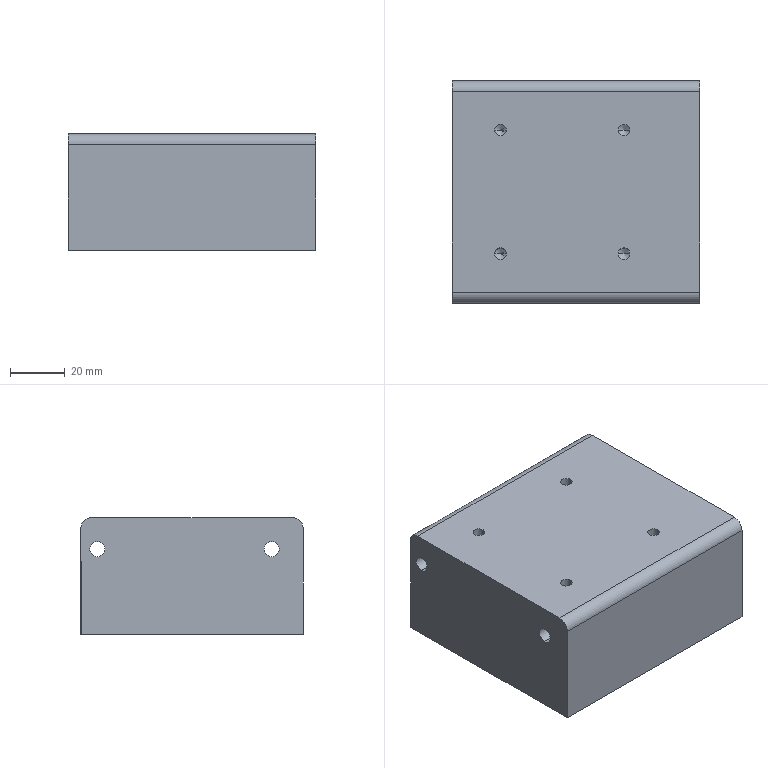Part | STEP file | FFH80-GY-003B^FFH85-PL-M75-B3-01_three-axis module | 1 solid | 45 faces | box 90 x 81 x 42.5 mm | volume 303221 mm3 | cylinder 23 | plane 12 | cone 10 | commonest cylinder face diameters 4.2 x8 5.5 x4 9 x4 2.5 x2 3 x2 8 x2
STEP:
#1=CARTESIAN_POINT('',(84.,34.5,14.25));
#2=VERTEX_POINT('',#1);
#3=CARTESIAN_POINT('',(84.,34.5,5.25));
#4=VERTEX_POINT('',#3);
#5=CARTESIAN_POINT('',(84.,34.5,9.75));
#6=DIRECTION('',(1.,0.,0.));
#7=DIRECTION('',(0.,0.,-1.));
#8=AXIS2_PLACEMENT_3D('',#5,#6,#7);
#9=CIRCLE('',#8,4.5);
#10=EDGE_CURVE('',#2,#4,#9,.T.);
#11=ORIENTED_EDGE('',*,*,#10,.F.);
#12=CARTESIAN_POINT('',(90.,34.5,14.25));
#13=VERTEX_POINT('',#12);
#14=CARTESIAN_POINT('',(90.,34.5,14.25));
#15=DIRECTION('',(1.,0.,0.));
#16=VECTOR('',#15,1000.);
#17=LINE('',#14,#16);
#18=EDGE_CURVE('',#2,#13,#17,.T.);
#19=ORIENTED_EDGE('',*,*,#18,.T.);
#20=CARTESIAN_POINT('',(90.,34.5,5.25));
#21=VERTEX_POINT('',#20);
#22=CARTESIAN_POINT('',(90.,34.5,9.75));
#23=DIRECTION('',(1.,0.,0.));
#24=DIRECTION('',(0.,0.,-1.));
#25=AXIS2_PLACEMENT_3D('',#22,#23,#24);
#26=CIRCLE('',#25,4.5);
#27=EDGE_CURVE('',#13,#21,#26,.T.);
#28=ORIENTED_EDGE('',*,*,#27,.T.);
#29=CARTESIAN_POINT('',(90.,34.5,5.25));
#30=DIRECTION('',(1.,0.,0.));
#31=VECTOR('',#30,1000.);
#32=LINE('',#29,#31);
#33=EDGE_CURVE('',#4,#21,#32,.T.);
#34=ORIENTED_EDGE('',*,*,#33,.F.);
#35=EDGE_LOOP('',(#11,#19,#28,#34));
#36=FACE_OUTER_BOUND('',#35,.T.);
#37=CARTESIAN_POINT('',(90.,34.5,9.75));
#38=DIRECTION('',(1.,0.,0.));
#39=DIRECTION('',(0.,0.,-1.));
#40=AXIS2_PLACEMENT_3D('',#37,#38,#39);
#41=CYLINDRICAL_SURFACE('',#40,4.5);
#42=ADVANCED_FACE('',(#36),#41,.F.);
#43=CARTESIAN_POINT('',(84.,-29.,14.25));
#44=VERTEX_POINT('',#43);
#45=CARTESIAN_POINT('',(84.,-29.,5.25));
#46=VERTEX_POINT('',#45);
#47=CARTESIAN_POINT('',(84.,-29.,9.75));
#48=DIRECTION('',(1.,0.,0.));
#49=DIRECTION('',(0.,0.,-1.));
#50=AXIS2_PLACEMENT_3D('',#47,#48,#49);
#51=CIRCLE('',#50,4.5);
#52=EDGE_CURVE('',#44,#46,#51,.T.);
#53=ORIENTED_EDGE('',*,*,#52,.F.);
#54=CARTESIAN_POINT('',(90.,-29.,14.25));
#55=VERTEX_POINT('',#54);
#56=CARTESIAN_POINT('',(90.,-29.,14.25));
#57=DIRECTION('',(1.,0.,0.));
#58=VECTOR('',#57,1000.);
#59=LINE('',#56,#58);
#60=EDGE_CURVE('',#44,#55,#59,.T.);
#61=ORIENTED_EDGE('',*,*,#60,.T.);
#62=CARTESIAN_POINT('',(90.,-29.,5.25));
#63=VERTEX_POINT('',#62);
#64=CARTESIAN_POINT('',(90.,-29.,9.75));
#65=DIRECTION('',(1.,0.,0.));
#66=DIRECTION('',(0.,0.,-1.));
#67=AXIS2_PLACEMENT_3D('',#64,#65,#66);
#68=CIRCLE('',#67,4.5);
#69=EDGE_CURVE('',#55,#63,#68,.T.);
#70=ORIENTED_EDGE('',*,*,#69,.T.);
#71=CARTESIAN_POINT('',(90.,-29.,5.25));
#72=DIRECTION('',(1.,0.,0.));
#73=VECTOR('',#72,1000.);
#74=LINE('',#71,#73);
#75=EDGE_CURVE('',#46,#63,#74,.T.);
#76=ORIENTED_EDGE('',*,*,#75,.F.);
#77=EDGE_LOOP('',(#53,#61,#70,#76));
#78=FACE_OUTER_BOUND('',#77,.T.);
#79=CARTESIAN_POINT('',(90.,-29.,9.75));
#80=DIRECTION('',(1.,0.,0.));
#81=DIRECTION('',(0.,0.,-1.));
#82=AXIS2_PLACEMENT_3D('',#79,#80,#81);
#83=CYLINDRICAL_SURFACE('',#82,4.5);
#84=ADVANCED_FACE('',(#78),#83,.F.);
#85=CARTESIAN_POINT('',(0.,34.5,12.5));
#86=VERTEX_POINT('',#85);
#87=CARTESIAN_POINT('',(0.,34.5,7.));
#88=VERTEX_POINT('',#87);
#89=CARTESIAN_POINT('',(0.,34.5,9.75));
#90=DIRECTION('',(1.,0.,0.));
#91=DIRECTION('',(0.,0.,-1.));
#92=AXIS2_PLACEMENT_3D('',#89,#90,#91);
#93=CIRCLE('',#92,2.75);
#94=EDGE_CURVE('',#86,#88,#93,.T.);
#95=ORIENTED_EDGE('',*,*,#94,.F.);
#96=CARTESIAN_POINT('',(84.,34.5,12.5));
#97=VERTEX_POINT('',#96);
#98=CARTESIAN_POINT('',(90.,34.5,12.5));
#99=DIRECTION('',(1.,0.,0.));
#100=VECTOR('',#99,1000.);
#101=LINE('',#98,#100);
#102=EDGE_CURVE('',#86,#97,#101,.T.);
#103=ORIENTED_EDGE('',*,*,#102,.T.);
#104=CARTESIAN_POINT('',(84.,34.5,7.));
#105=VERTEX_POINT('',#104);
#106=CARTESIAN_POINT('',(84.,34.5,9.75));
#107=DIRECTION('',(-1.,0.,0.));
#108=DIRECTION('',(0.,0.,-1.));
#109=AXIS2_PLACEMENT_3D('',#106,#107,#108);
#110=CIRCLE('',#109,2.75);
#111=EDGE_CURVE('',#105,#97,#110,.T.);
#112=ORIENTED_EDGE('',*,*,#111,.F.);
#113=CARTESIAN_POINT('',(90.,34.5,7.));
#114=DIRECTION('',(1.,0.,0.));
#115=VECTOR('',#114,1000.);
#116=LINE('',#113,#115);
#117=EDGE_CURVE('',#88,#105,#116,.T.);
#118=ORIENTED_EDGE('',*,*,#117,.F.);
#119=EDGE_LOOP('',(#95,#103,#112,#118));
#120=FACE_OUTER_BOUND('',#119,.T.);
#121=CARTESIAN_POINT('',(90.,34.5,9.75));
#122=DIRECTION('',(1.,0.,0.));
#123=DIRECTION('',(0.,0.,-1.));
#124=AXIS2_PLACEMENT_3D('',#121,#122,#123);
#125=CYLINDRICAL_SURFACE('',#124,2.75);
#126=ADVANCED_FACE('',(#120),#125,.F.);
#127=CARTESIAN_POINT('',(0.,-29.,12.5));
#128=VERTEX_POINT('',#127);
#129=CARTESIAN_POINT('',(0.,-29.,7.));
#130=VERTEX_POINT('',#129);
#131=CARTESIAN_POINT('',(0.,-29.,9.75));
#132=DIRECTION('',(1.,0.,0.));
#133=DIRECTION('',(0.,0.,-1.));
#134=AXIS2_PLACEMENT_3D('',#131,#132,#133);
#135=CIRCLE('',#134,2.75);
#136=EDGE_CURVE('',#128,#130,#135,.T.);
#137=ORIENTED_EDGE('',*,*,#136,.F.);
#138=CARTESIAN_POINT('',(84.,-29.,12.5));
#139=VERTEX_POINT('',#138);
#140=CARTESIAN_POINT('',(90.,-29.,12.5));
#141=DIRECTION('',(1.,0.,0.));
#142=VECTOR('',#141,1000.);
#143=LINE('',#140,#142);
#144=EDGE_CURVE('',#128,#139,#143,.T.);
#145=ORIENTED_EDGE('',*,*,#144,.T.);
#146=CARTESIAN_POINT('',(84.,-29.,7.));
#147=VERTEX_POINT('',#146);
#148=CARTESIAN_POINT('',(84.,-29.,9.75));
#149=DIRECTION('',(-1.,0.,0.));
#150=DIRECTION('',(0.,0.,-1.));
#151=AXIS2_PLACEMENT_3D('',#148,#149,#150);
#152=CIRCLE('',#151,2.75);
#153=EDGE_CURVE('',#147,#139,#152,.T.);
#154=ORIENTED_EDGE('',*,*,#153,.F.);
#155=CARTESIAN_POINT('',(90.,-29.,7.));
#156=DIRECTION('',(1.,0.,0.));
#157=VECTOR('',#156,1000.);
#158=LINE('',#155,#157);
#159=EDGE_CURVE('',#130,#147,#158,.T.);
#160=ORIENTED_EDGE('',*,*,#159,.F.);
#161=EDGE_LOOP('',(#137,#145,#154,#160));
#162=FACE_OUTER_BOUND('',#161,.T.);
#163=CARTESIAN_POINT('',(90.,-29.,9.75));
#164=DIRECTION('',(1.,0.,0.));
#165=DIRECTION('',(0.,0.,-1.));
#166=AXIS2_PLACEMENT_3D('',#163,#164,#165);
#167=CYLINDRICAL_SURFACE('',#166,2.75);
#168=ADVANCED_FACE('',(#162),#167,.F.);
#169=CARTESIAN_POINT('',(6.,34.2,-6.75));
#170=VERTEX_POINT('',#169);
#171=CARTESIAN_POINT('',(6.,34.2,-3.75));
#172=VERTEX_POINT('',#171);
#173=CARTESIAN_POINT('',(6.,34.2,-5.25));
#174=DIRECTION('',(0.,1.,0.));
#175=DIRECTION('',(0.,0.,1.));
#176=AXIS2_PLACEMENT_3D('',#173,#174,#175);
#177=CIRCLE('',#176,1.5);
#178=EDGE_CURVE('',#170,#172,#177,.T.);
#179=ORIENTED_EDGE('',*,*,#178,.F.);
#180=CARTESIAN_POINT('',(6.,40.2,-6.75));
#181=VERTEX_POINT('',#180);
#182=CARTESIAN_POINT('',(6.,40.2,-6.75));
#183=DIRECTION('',(0.,1.,0.));
#184=VECTOR('',#183,1000.);
#185=LINE('',#182,#184);
#186=EDGE_CURVE('',#170,#181,#185,.T.);
#187=ORIENTED_EDGE('',*,*,#186,.T.);
#188=CARTESIAN_POINT('',(6.,40.2,-3.75));
#189=VERTEX_POINT('',#188);
#190=CARTESIAN_POINT('',(6.,40.2,-5.25));
#191=DIRECTION('',(0.,-1.,0.));
#192=DIRECTION('',(0.,0.,1.));
#193=AXIS2_PLACEMENT_3D('',#190,#191,#192);
#194=CIRCLE('',#193,1.5);
#195=EDGE_CURVE('',#189,#181,#194,.T.);
#196=ORIENTED_EDGE('',*,*,#195,.F.);
#197=CARTESIAN_POINT('',(6.,40.2,-3.75));
#198=DIRECTION('',(0.,1.,0.));
#199=VECTOR('',#198,1000.);
#200=LINE('',#197,#199);
#201=EDGE_CURVE('',#172,#189,#200,.T.);
#202=ORIENTED_EDGE('',*,*,#201,.F.);
#203=EDGE_LOOP('',(#179,#187,#196,#202));
#204=FACE_OUTER_BOUND('',#203,.T.);
#205=CARTESIAN_POINT('',(6.,40.2,-5.25));
#206=DIRECTION('',(0.,1.,0.));
#207=DIRECTION('',(0.,0.,1.));
#208=AXIS2_PLACEMENT_3D('',#205,#206,#207);
#209=CYLINDRICAL_SURFACE('',#208,1.5);
#210=ADVANCED_FACE('',(#204),#209,.F.);
#211=CARTESIAN_POINT('',(60.4,22.5,2.25));
#212=VERTEX_POINT('',#211);
#213=CARTESIAN_POINT('',(64.6,22.5,2.25));
#214=VERTEX_POINT('',#213);
#215=CARTESIAN_POINT('',(62.5,22.5,2.25));
#216=DIRECTION('',(0.,0.,1.));
#217=DIRECTION('',(1.,0.,0.));
#218=AXIS2_PLACEMENT_3D('',#215,#216,#217);
#219=CIRCLE('',#218,2.1);
#220=EDGE_CURVE('',#212,#214,#219,.T.);
#221=ORIENTED_EDGE('',*,*,#220,.F.);
#222=CARTESIAN_POINT('',(60.4,22.5,21.25));
#223=VERTEX_POINT('',#222);
#224=CARTESIAN_POINT('',(60.4,22.5,21.25));
#225=DIRECTION('',(0.,0.,1.));
#226=VECTOR('',#225,1000.);
#227=LINE('',#224,#226);
#228=EDGE_CURVE('',#212,#223,#227,.T.);
#229=ORIENTED_EDGE('',*,*,#228,.T.);
#230=CARTESIAN_POINT('',(64.6,22.5,21.25));
#231=VERTEX_POINT('',#230);
#232=CARTESIAN_POINT('',(62.5,22.5,21.25));
#233=DIRECTION('',(0.,0.,1.));
#234=DIRECTION('',(1.,0.,0.));
#235=AXIS2_PLACEMENT_3D('',#232,#233,#234);
#236=CIRCLE('',#235,2.1);
#237=EDGE_CURVE('',#223,#231,#236,.T.);
#238=ORIENTED_EDGE('',*,*,#237,.T.);
#239=CARTESIAN_POINT('',(64.6,22.5,21.25));
#240=DIRECTION('',(0.,0.,1.));
#241=VECTOR('',#240,1000.);
#242=LINE('',#239,#241);
#243=EDGE_CURVE('',#214,#231,#242,.T.);
#244=ORIENTED_EDGE('',*,*,#243,.F.);
#245=EDGE_LOOP('',(#221,#229,#238,#244));
#246=FACE_OUTER_BOUND('',#245,.T.);
#247=CARTESIAN_POINT('',(62.5,22.5,21.25));
#248=DIRECTION('',(0.,0.,1.));
#249=DIRECTION('',(1.,0.,0.));
#250=AXIS2_PLACEMENT_3D('',#247,#248,#249);
#251=CYLINDRICAL_SURFACE('',#250,2.1);
#252=ADVANCED_FACE('',(#246),#251,.F.);
#253=CARTESIAN_POINT('',(15.4,22.5,2.25));
#254=VERTEX_POINT('',#253);
#255=CARTESIAN_POINT('',(19.6,22.5,2.25));
#256=VERTEX_POINT('',#255);
#257=CARTESIAN_POINT('',(17.5,22.5,2.25));
#258=DIRECTION('',(0.,0.,1.));
#259=DIRECTION('',(1.,0.,0.));
#260=AXIS2_PLACEMENT_3D('',#257,#258,#259);
#261=CIRCLE('',#260,2.1);
#262=EDGE_CURVE('',#254,#256,#261,.T.);
#263=ORIENTED_EDGE('',*,*,#262,.F.);
#264=CARTESIAN_POINT('',(15.4,22.5,21.25));
#265=VERTEX_POINT('',#264);
#266=CARTESIAN_POINT('',(15.4,22.5,21.25));
#267=DIRECTION('',(0.,0.,1.));
#268=VECTOR('',#267,1000.);
#269=LINE('',#266,#268);
#270=EDGE_CURVE('',#254,#265,#269,.T.);
#271=ORIENTED_EDGE('',*,*,#270,.T.);
#272=CARTESIAN_POINT('',(19.6,22.5,21.25));
#273=VERTEX_POINT('',#272);
#274=CARTESIAN_POINT('',(17.5,22.5,21.25));
#275=DIRECTION('',(0.,0.,1.));
#276=DIRECTION('',(1.,0.,0.));
#277=AXIS2_PLACEMENT_3D('',#274,#275,#276);
#278=CIRCLE('',#277,2.1);
#279=EDGE_CURVE('',#265,#273,#278,.T.);
#280=ORIENTED_EDGE('',*,*,#279,.T.);
#281=CARTESIAN_POINT('',(19.6,22.5,21.25));
#282=DIRECTION('',(0.,0.,1.));
#283=VECTOR('',#282,1000.);
#284=LINE('',#281,#283);
#285=EDGE_CURVE('',#256,#273,#284,.T.);
#286=ORIENTED_EDGE('',*,*,#285,.F.);
#287=EDGE_LOOP('',(#263,#271,#280,#286));
#288=FACE_OUTER_BOUND('',#287,.T.);
#289=CARTESIAN_POINT('',(17.5,22.5,21.25));
#290=DIRECTION('',(0.,0.,1.));
#291=DIRECTION('',(1.,0.,0.));
#292=AXIS2_PLACEMENT_3D('',#289,#290,#291);
#293=CYLINDRICAL_SURFACE('',#292,2.1);
#294=ADVANCED_FACE('',(#288),#293,.F.);
#295=CARTESIAN_POINT('',(60.4,-22.5,2.25));
#296=VERTEX_POINT('',#295);
#297=CARTESIAN_POINT('',(64.6,-22.5,2.25));
#298=VERTEX_POINT('',#297);
#299=CARTESIAN_POINT('',(62.5,-22.5,2.25));
#300=DIRECTION('',(0.,0.,1.));
#301=DIRECTION('',(1.,0.,0.));
#302=AXIS2_PLACEMENT_3D('',#299,#300,#301);
#303=CIRCLE('',#302,2.1);
#304=EDGE_CURVE('',#296,#298,#303,.T.);
#305=ORIENTED_EDGE('',*,*,#304,.F.);
#306=CARTESIAN_POINT('',(60.4,-22.5,21.25));
#307=VERTEX_POINT('',#306);
#308=CARTESIAN_POINT('',(60.4,-22.5,21.25));
#309=DIRECTION('',(0.,0.,1.));
#310=VECTOR('',#309,1000.);
#311=LINE('',#308,#310);
#312=EDGE_CURVE('',#296,#307,#311,.T.);
#313=ORIENTED_EDGE('',*,*,#312,.T.);
#314=CARTESIAN_POINT('',(64.6,-22.5,21.25));
#315=VERTEX_POINT('',#314);
#316=CARTESIAN_POINT('',(62.5,-22.5,21.25));
#317=DIRECTION('',(0.,0.,1.));
#318=DIRECTION('',(1.,0.,0.));
#319=AXIS2_PLACEMENT_3D('',#316,#317,#318);
#320=CIRCLE('',#319,2.1);
#321=EDGE_CURVE('',#307,#315,#320,.T.);
#322=ORIENTED_EDGE('',*,*,#321,.T.);
#323=CARTESIAN_POINT('',(64.6,-22.5,21.25));
#324=DIRECTION('',(0.,0.,1.));
#325=VECTOR('',#324,1000.);
#326=LINE('',#323,#325);
#327=EDGE_CURVE('',#298,#315,#326,.T.);
#328=ORIENTED_EDGE('',*,*,#327,.F.);
#329=EDGE_LOOP('',(#305,#313,#322,#328));
#330=FACE_OUTER_BOUND('',#329,.T.);
#331=CARTESIAN_POINT('',(62.5,-22.5,21.25));
#332=DIRECTION('',(0.,0.,1.));
#333=DIRECTION('',(1.,0.,0.));
#334=AXIS2_PLACEMENT_3D('',#331,#332,#333);
#335=CYLINDRICAL_SURFACE('',#334,2.1);
#336=ADVANCED_FACE('',(#330),#335,.F.);
#337=CARTESIAN_POINT('',(15.4,-22.5,2.25));
#338=VERTEX_POINT('',#337);
#339=CARTESIAN_POINT('',(19.6,-22.5,2.25));
#340=VERTEX_POINT('',#339);
#341=CARTESIAN_POINT('',(17.5,-22.5,2.25));
#342=DIRECTION('',(0.,0.,1.));
#343=DIRECTION('',(1.,0.,0.));
#344=AXIS2_PLACEMENT_3D('',#341,#342,#343);
#345=CIRCLE('',#344,2.1);
#346=EDGE_CURVE('',#338,#340,#345,.T.);
#347=ORIENTED_EDGE('',*,*,#346,.F.);
#348=CARTESIAN_POINT('',(15.4,-22.5,21.25));
#349=VERTEX_POINT('',#348);
#350=CARTESIAN_POINT('',(15.4,-22.5,21.25));
#351=DIRECTION('',(0.,0.,1.));
#352=VECTOR('',#351,1000.);
#353=LINE('',#350,#352);
#354=EDGE_CURVE('',#338,#349,#353,.T.);
#355=ORIENTED_EDGE('',*,*,#354,.T.);
#356=CARTESIAN_POINT('',(19.6,-22.5,21.25));
#357=VERTEX_POINT('',#356);
#358=CARTESIAN_POINT('',(17.5,-22.5,21.25));
#359=DIRECTION('',(0.,0.,1.));
#360=DIRECTION('',(1.,0.,0.));
#361=AXIS2_PLACEMENT_3D('',#358,#359,#360);
#362=CIRCLE('',#361,2.1);
#363=EDGE_CURVE('',#349,#357,#362,.T.);
#364=ORIENTED_EDGE('',*,*,#363,.T.);
#365=CARTESIAN_POINT('',(19.6,-22.5,21.25));
#366=DIRECTION('',(0.,0.,1.));
#367=VECTOR('',#366,1000.);
#368=LINE('',#365,#367);
#369=EDGE_CURVE('',#340,#357,#368,.T.);
#370=ORIENTED_EDGE('',*,*,#369,.F.);
#371=EDGE_LOOP('',(#347,#355,#364,#370));
#372=FACE_OUTER_BOUND('',#371,.T.);
#373=CARTESIAN_POINT('',(17.5,-22.5,21.25));
#374=DIRECTION('',(0.,0.,1.));
#375=DIRECTION('',(1.,0.,0.));
#376=AXIS2_PLACEMENT_3D('',#373,#374,#375);
#377=CYLINDRICAL_SURFACE('',#376,2.1);
#378=ADVANCED_FACE('',(#372),#377,.F.);
#379=CARTESIAN_POINT('',(62.5,22.5,0.9882));
#380=VERTEX_POINT('',#379);
#381=CARTESIAN_POINT('',(64.6,22.5,2.25));
#382=DIRECTION('',(0.8572,0.,0.515));
#383=VECTOR('',#382,1000.);
#384=LINE('',#381,#383);
#385=EDGE_CURVE('',#380,#214,#384,.T.);
#386=ORIENTED_EDGE('',*,*,#385,.F.);
#387=CARTESIAN_POINT('',(60.4,22.5,2.25));
#388=DIRECTION('',(-0.8572,0.,0.515));
#389=VECTOR('',#388,1000.);
#390=LINE('',#387,#389);
#391=EDGE_CURVE('',#380,#212,#390,.T.);
#392=ORIENTED_EDGE('',*,*,#391,.T.);
#393=ORIENTED_EDGE('',*,*,#220,.T.);
#394=EDGE_LOOP('',(#386,#392,#393));
#395=FACE_OUTER_BOUND('',#394,.T.);
#396=CARTESIAN_POINT('',(62.5,22.5,2.25));
#397=DIRECTION('',(0.,0.,1.));
#398=DIRECTION('',(1.,0.,0.));
#399=AXIS2_PLACEMENT_3D('',#396,#397,#398);
#400=CONICAL_SURFACE('',#399,2.1,1.03);
#401=ADVANCED_FACE('',(#395),#400,.F.);
#402=CARTESIAN_POINT('',(17.5,22.5,0.9882));
#403=VERTEX_POINT('',#402);
#404=CARTESIAN_POINT('',(19.6,22.5,2.25));
#405=DIRECTION('',(0.8572,0.,0.515));
#406=VECTOR('',#405,1000.);
#407=LINE('',#404,#406);
#408=EDGE_CURVE('',#403,#256,#407,.T.);
#409=ORIENTED_EDGE('',*,*,#408,.F.);
#410=CARTESIAN_POINT('',(15.4,22.5,2.25));
#411=DIRECTION('',(-0.8572,0.,0.515));
#412=VECTOR('',#411,1000.);
#413=LINE('',#410,#412);
#414=EDGE_CURVE('',#403,#254,#413,.T.);
#415=ORIENTED_EDGE('',*,*,#414,.T.);
#416=ORIENTED_EDGE('',*,*,#262,.T.);
#417=EDGE_LOOP('',(#409,#415,#416));
#418=FACE_OUTER_BOUND('',#417,.T.);
#419=CARTESIAN_POINT('',(17.5,22.5,2.25));
#420=DIRECTION('',(0.,0.,1.));
#421=DIRECTION('',(1.,0.,0.));
#422=AXIS2_PLACEMENT_3D('',#419,#420,#421);
#423=CONICAL_SURFACE('',#422,2.1,1.03);
#424=ADVANCED_FACE('',(#418),#423,.F.);
#425=CARTESIAN_POINT('',(62.5,-22.5,0.9882));
#426=VERTEX_POINT('',#425);
#427=CARTESIAN_POINT('',(64.6,-22.5,2.25));
#428=DIRECTION('',(0.8572,0.,0.515));
#429=VECTOR('',#428,1000.);
#430=LINE('',#427,#429);
#431=EDGE_CURVE('',#426,#298,#430,.T.);
#432=ORIENTED_EDGE('',*,*,#431,.F.);
#433=CARTESIAN_POINT('',(60.4,-22.5,2.25));
#434=DIRECTION('',(-0.8572,0.,0.515));
#435=VECTOR('',#434,1000.);
#436=LINE('',#433,#435);
#437=EDGE_CURVE('',#426,#296,#436,.T.);
#438=ORIENTED_EDGE('',*,*,#437,.T.);
#439=ORIENTED_EDGE('',*,*,#304,.T.);
#440=EDGE_LOOP('',(#432,#438,#439));
#441=FACE_OUTER_BOUND('',#440,.T.);
#442=CARTESIAN_POINT('',(62.5,-22.5,2.25));
#443=DIRECTION('',(0.,0.,1.));
#444=DIRECTION('',(1.,0.,0.));
#445=AXIS2_PLACEMENT_3D('',#442,#443,#444);
#446=CONICAL_SURFACE('',#445,2.1,1.03);
#447=ADVANCED_FACE('',(#441),#446,.F.);
#448=CARTESIAN_POINT('',(17.5,-22.5,0.9882));
#449=VERTEX_POINT('',#448);
#450=CARTESIAN_POINT('',(19.6,-22.5,2.25));
#451=DIRECTION('',(0.8572,0.,0.515));
#452=VECTOR('',#451,1000.);
#453=LINE('',#450,#452);
#454=EDGE_CURVE('',#449,#340,#453,.T.);
#455=ORIENTED_EDGE('',*,*,#454,.F.);
#456=CARTESIAN_POINT('',(15.4,-22.5,2.25));
#457=DIRECTION('',(-0.8572,0.,0.515));
#458=VECTOR('',#457,1000.);
#459=LINE('',#456,#458);
#460=EDGE_CURVE('',#449,#338,#459,.T.);
#461=ORIENTED_EDGE('',*,*,#460,.T.);
#462=ORIENTED_EDGE('',*,*,#346,.T.);
#463=EDGE_LOOP('',(#455,#461,#462));
#464=FACE_OUTER_BOUND('',#463,.T.);
#465=CARTESIAN_POINT('',(17.5,-22.5,2.25));
#466=DIRECTION('',(0.,0.,1.));
#467=DIRECTION('',(1.,0.,0.));
#468=AXIS2_PLACEMENT_3D('',#465,#466,#467);
#469=CONICAL_SURFACE('',#468,2.1,1.03);
#470=ADVANCED_FACE('',(#464),#469,.F.);
#471=CARTESIAN_POINT('',(6.,31.7,-6.5));
#472=VERTEX_POINT('',#471);
#473=CARTESIAN_POINT('',(6.,31.7,-4.));
#474=VERTEX_POINT('',#473);
#475=CARTESIAN_POINT('',(6.,31.7,-5.25));
#476=DIRECTION('',(0.,1.,0.));
#477=DIRECTION('',(0.,0.,1.));
#478=AXIS2_PLACEMENT_3D('',#475,#476,#477);
#479=CIRCLE('',#478,1.25);
#480=EDGE_CURVE('',#472,#474,#479,.T.);
#481=ORIENTED_EDGE('',*,*,#480,.F.);
#482=CARTESIAN_POINT('',(6.,34.2,-6.5));
#483=VERTEX_POINT('',#482);
#484=CARTESIAN_POINT('',(6.,40.2,-6.5));
#485=DIRECTION('',(0.,1.,0.));
#486=VECTOR('',#485,1000.);
#487=LINE('',#484,#486);
#488=EDGE_CURVE('',#472,#483,#487,.T.);
#489=ORIENTED_EDGE('',*,*,#488,.T.);
#490=CARTESIAN_POINT('',(6.,34.2,-4.));
#491=VERTEX_POINT('',#490);
#492=CARTESIAN_POINT('',(6.,34.2,-5.25));
#493=DIRECTION('',(0.,1.,0.));
#494=DIRECTION('',(0.,0.,1.));
#495=AXIS2_PLACEMENT_3D('',#492,#493,#494);
#496=CIRCLE('',#495,1.25);
#497=EDGE_CURVE('',#483,#491,#496,.T.);
#498=ORIENTED_EDGE('',*,*,#497,.T.);
#499=CARTESIAN_POINT('',(6.,40.2,-4.));
#500=DIRECTION('',(0.,1.,0.));
#501=VECTOR('',#500,1000.);
#502=LINE('',#499,#501);
#503=EDGE_CURVE('',#474,#491,#502,.T.);
#504=ORIENTED_EDGE('',*,*,#503,.F.);
#505=EDGE_LOOP('',(#481,#489,#498,#504));
#506=FACE_OUTER_BOUND('',#505,.T.);
#507=CARTESIAN_POINT('',(6.,40.2,-5.25));
#508=DIRECTION('',(0.,1.,0.));
#509=DIRECTION('',(0.,0.,1.));
#510=AXIS2_PLACEMENT_3D('',#507,#508,#509);
#511=CYLINDRICAL_SURFACE('',#510,1.25);
#512=ADVANCED_FACE('',(#506),#511,.F.);
#513=CARTESIAN_POINT('',(6.,30.949,-5.25));
#514=VERTEX_POINT('',#513);
#515=CARTESIAN_POINT('',(6.,31.7,-4.));
#516=DIRECTION('',(0.,0.515,0.8572));
#517=VECTOR('',#516,1000.);
#518=LINE('',#515,#517);
#519=EDGE_CURVE('',#514,#474,#518,.T.);
#520=ORIENTED_EDGE('',*,*,#519,.F.);
#521=CARTESIAN_POINT('',(6.,31.7,-6.5));
#522=DIRECTION('',(0.,0.515,-0.8572));
#523=VECTOR('',#522,1000.);
#524=LINE('',#521,#523);
#525=EDGE_CURVE('',#514,#472,#524,.T.);
#526=ORIENTED_EDGE('',*,*,#525,.T.);
#527=ORIENTED_EDGE('',*,*,#480,.T.);
#528=EDGE_LOOP('',(#520,#526,#527));
#529=FACE_OUTER_BOUND('',#528,.T.);
#530=CARTESIAN_POINT('',(6.,31.7,-5.25));
#531=DIRECTION('',(0.,1.,0.));
#532=DIRECTION('',(0.,0.,1.));
#533=AXIS2_PLACEMENT_3D('',#530,#531,#532);
#534=CONICAL_SURFACE('',#533,1.25,1.03);
#535=ADVANCED_FACE('',(#529),#534,.F.);
#536=CARTESIAN_POINT('',(90.,40.5,-21.25));
#537=VERTEX_POINT('',#536);
#538=CARTESIAN_POINT('',(12.5,40.5,-21.25));
#539=VERTEX_POINT('',#538);
#540=CARTESIAN_POINT('',(90.,40.5,-21.25));
#541=DIRECTION('',(-1.,0.,0.));
#542=VECTOR('',#541,1000.);
#543=LINE('',#540,#542);
#544=EDGE_CURVE('',#537,#539,#543,.T.);
#545=ORIENTED_EDGE('',*,*,#544,.F.);
#546=CARTESIAN_POINT('',(90.,-40.5,-21.25));
#547=VERTEX_POINT('',#546);
#548=CARTESIAN_POINT('',(90.,40.5,-21.25));
#549=DIRECTION('',(0.,1.,0.));
#550=VECTOR('',#549,1000.);
#551=LINE('',#548,#550);
#552=EDGE_CURVE('',#547,#537,#551,.T.);
#553=ORIENTED_EDGE('',*,*,#552,.F.);
#554=CARTESIAN_POINT('',(0.,-40.5,-21.25));
#555=VERTEX_POINT('',#554);
#556=CARTESIAN_POINT('',(90.,-40.5,-21.25));
#557=DIRECTION('',(1.,0.,0.));
#558=VECTOR('',#557,1000.);
#559=LINE('',#556,#558);
#560=EDGE_CURVE('',#555,#547,#559,.T.);
#561=ORIENTED_EDGE('',*,*,#560,.F.);
#562=CARTESIAN_POINT('',(0.,40.2,-21.25));
#563=VERTEX_POINT('',#562);
#564=CARTESIAN_POINT('',(0.,40.5,-21.25));
#565=DIRECTION('',(0.,-1.,0.));
#566=VECTOR('',#565,1000.);
#567=LINE('',#564,#566);
#568=EDGE_CURVE('',#563,#555,#567,.T.);
#569=ORIENTED_EDGE('',*,*,#568,.F.);
#570=CARTESIAN_POINT('',(12.5,40.2,-21.25));
#571=VERTEX_POINT('',#570);
#572=CARTESIAN_POINT('',(90.,40.2,-21.25));
#573=DIRECTION('',(-1.,0.,0.));
#574=VECTOR('',#573,1000.);
#575=LINE('',#572,#574);
#576=EDGE_CURVE('',#571,#563,#575,.T.);
#577=ORIENTED_EDGE('',*,*,#576,.F.);
#578=CARTESIAN_POINT('',(12.5,40.2,-21.25));
#579=DIRECTION('',(0.,1.,0.));
#580=VECTOR('',#579,1000.);
#581=LINE('',#578,#580);
#582=EDGE_CURVE('',#571,#539,#581,.T.);
#583=ORIENTED_EDGE('',*,*,#582,.T.);
#584=EDGE_LOOP('',(#545,#553,#561,#569,#577,#583));
#585=FACE_OUTER_BOUND('',#584,.T.);
#586=CARTESIAN_POINT('',(90.,40.5,-21.25));
#587=DIRECTION('',(0.,0.,1.));
#588=DIRECTION('',(0.,-1.,0.));
#589=AXIS2_PLACEMENT_3D('',#586,#587,#588);
#590=PLANE('',#589);
#591=ADVANCED_FACE('',(#585),#590,.F.);
#592=CARTESIAN_POINT('',(90.,40.5,17.25));
#593=VERTEX_POINT('',#592);
#594=CARTESIAN_POINT('',(90.,40.5,-21.25));
#595=DIRECTION('',(0.,0.,1.));
#596=VECTOR('',#595,1000.);
#597=LINE('',#594,#596);
#598=EDGE_CURVE('',#537,#593,#597,.T.);
#599=ORIENTED_EDGE('',*,*,#598,.F.);
#600=ORIENTED_EDGE('',*,*,#544,.T.);
#601=CARTESIAN_POINT('',(12.5,40.5,3.25));
#602=VERTEX_POINT('',#601);
#603=CARTESIAN_POINT('',(12.5,40.5,-21.25));
#604=DIRECTION('',(0.,0.,-1.));
#605=VECTOR('',#604,1000.);
#606=LINE('',#603,#605);
#607=EDGE_CURVE('',#602,#539,#606,.T.);
#608=ORIENTED_EDGE('',*,*,#607,.F.);
#609=CARTESIAN_POINT('',(10.5,40.5,5.25));
#610=VERTEX_POINT('',#609);
#611=CARTESIAN_POINT('',(10.5,40.5,3.25));
#612=DIRECTION('',(0.,1.,0.));
#613=DIRECTION('',(0.,0.,-1.));
#614=AXIS2_PLACEMENT_3D('',#611,#612,#613);
#615=CIRCLE('',#614,2.);
#616=EDGE_CURVE('',#610,#602,#615,.T.);
#617=ORIENTED_EDGE('',*,*,#616,.F.);
#618=CARTESIAN_POINT('',(0.,40.5,5.25));
#619=VERTEX_POINT('',#618);
#620=CARTESIAN_POINT('',(90.,40.5,5.25));
#621=DIRECTION('',(1.,0.,0.));
#622=VECTOR('',#621,1000.);
#623=LINE('',#620,#622);
#624=EDGE_CURVE('',#619,#610,#623,.T.);
#625=ORIENTED_EDGE('',*,*,#624,.F.);
#626=CARTESIAN_POINT('',(0.,40.5,17.25));
#627=VERTEX_POINT('',#626);
#628=CARTESIAN_POINT('',(0.,40.5,-21.25));
#629=DIRECTION('',(0.,0.,-1.));
#630=VECTOR('',#629,1000.);
#631=LINE('',#628,#630);
#632=EDGE_CURVE('',#627,#619,#631,.T.);
#633=ORIENTED_EDGE('',*,*,#632,.F.);
#634=CARTESIAN_POINT('',(90.,40.5,17.25));
#635=DIRECTION('',(-1.,0.,0.));
#636=VECTOR('',#635,1000.);
#637=LINE('',#634,#636);
#638=EDGE_CURVE('',#593,#627,#637,.T.);
#639=ORIENTED_EDGE('',*,*,#638,.F.);
#640=EDGE_LOOP('',(#599,#600,#608,#617,#625,#633,#639));
#641=FACE_OUTER_BOUND('',#640,.T.);
#642=CARTESIAN_POINT('',(90.,40.5,-21.25));
#643=DIRECTION('',(0.,-1.,0.));
#644=DIRECTION('',(0.,0.,-1.));
#645=AXIS2_PLACEMENT_3D('',#642,#643,#644);
#646=PLANE('',#645);
#647=ADVANCED_FACE('',(#641),#646,.F.);
#648=CARTESIAN_POINT('',(90.,34.5,9.75));
#649=DIRECTION('',(1.,0.,0.));
#650=DIRECTION('',(0.,0.,-1.));
#651=AXIS2_PLACEMENT_3D('',#648,#649,#650);
#652=CIRCLE('',#651,4.5);
#653=EDGE_CURVE('',#21,#13,#652,.T.);
#654=ORIENTED_EDGE('',*,*,#653,.F.);
#655=ORIENTED_EDGE('',*,*,#27,.F.);
#656=EDGE_LOOP('',(#654,#655));
#657=FACE_BOUND('',#656,.T.);
#658=CARTESIAN_POINT('',(90.,-29.,9.75));
#659=DIRECTION('',(1.,0.,0.));
#660=DIRECTION('',(0.,0.,-1.));
#661=AXIS2_PLACEMENT_3D('',#658,#659,#660);
#662=CIRCLE('',#661,4.5);
#663=EDGE_CURVE('',#63,#55,#662,.T.);
#664=ORIENTED_EDGE('',*,*,#663,.F.);
#665=ORIENTED_EDGE('',*,*,#69,.F.);
#666=EDGE_LOOP('',(#664,#665));
#667=FACE_BOUND('',#666,.T.);
#668=CARTESIAN_POINT('',(90.,-40.5,17.25));
#669=VERTEX_POINT('',#668);
#670=CARTESIAN_POINT('',(90.,-40.5,0.));
#671=DIRECTION('',(0.,0.,1.));
#672=VECTOR('',#671,1000.);
#673=LINE('',#670,#672);
#674=EDGE_CURVE('',#547,#669,#673,.T.);
#675=ORIENTED_EDGE('',*,*,#674,.F.);
#676=ORIENTED_EDGE('',*,*,#552,.T.);
#677=ORIENTED_EDGE('',*,*,#598,.T.);
#678=CARTESIAN_POINT('',(90.,36.5,21.25));
#679=VERTEX_POINT('',#678);
#680=CARTESIAN_POINT('',(90.,36.5,17.25));
#681=DIRECTION('',(-1.,0.,0.));
#682=DIRECTION('',(0.,0.,1.));
#683=AXIS2_PLACEMENT_3D('',#680,#681,#682);
#684=CIRCLE('',#683,4.);
#685=EDGE_CURVE('',#679,#593,#684,.T.);
#686=ORIENTED_EDGE('',*,*,#685,.F.);
#687=CARTESIAN_POINT('',(90.,-36.5,21.25));
#688=VERTEX_POINT('',#687);
#689=CARTESIAN_POINT('',(90.,0.,21.25));
#690=DIRECTION('',(0.,1.,0.));
#691=VECTOR('',#690,1000.);
#692=LINE('',#689,#691);
#693=EDGE_CURVE('',#688,#679,#692,.T.);
#694=ORIENTED_EDGE('',*,*,#693,.F.);
#695=CARTESIAN_POINT('',(90.,-36.5,17.25));
#696=DIRECTION('',(-1.,0.,0.));
#697=DIRECTION('',(0.,0.,1.));
#698=AXIS2_PLACEMENT_3D('',#695,#696,#697);
#699=CIRCLE('',#698,4.);
#700=EDGE_CURVE('',#669,#688,#699,.T.);
#701=ORIENTED_EDGE('',*,*,#700,.F.);
#702=EDGE_LOOP('',(#675,#676,#677,#686,#694,#701));
#703=FACE_OUTER_BOUND('',#702,.T.);
#704=CARTESIAN_POINT('',(90.,0.,0.));
#705=DIRECTION('',(-1.,0.,0.));
#706=DIRECTION('',(0.,0.,1.));
#707=AXIS2_PLACEMENT_3D('',#704,#705,#706);
#708=PLANE('',#707);
#709=ADVANCED_FACE('',(#657,#667,#703),#708,.F.);
#710=CARTESIAN_POINT('',(0.,-40.5,17.25));
#711=VERTEX_POINT('',#710);
#712=CARTESIAN_POINT('',(0.,-40.5,-21.25));
#713=DIRECTION('',(0.,0.,1.));
#714=VECTOR('',#713,1000.);
#715=LINE('',#712,#714);
#716=EDGE_CURVE('',#555,#711,#715,.T.);
#717=ORIENTED_EDGE('',*,*,#716,.F.);
#718=ORIENTED_EDGE('',*,*,#560,.T.);
#719=ORIENTED_EDGE('',*,*,#674,.T.);
#720=CARTESIAN_POINT('',(90.,-40.5,17.25));
#721=DIRECTION('',(1.,0.,0.));
#722=VECTOR('',#721,1000.);
#723=LINE('',#720,#722);
#724=EDGE_CURVE('',#711,#669,#723,.T.);
#725=ORIENTED_EDGE('',*,*,#724,.F.);
#726=EDGE_LOOP('',(#717,#718,#719,#725));
#727=FACE_OUTER_BOUND('',#726,.T.);
#728=CARTESIAN_POINT('',(90.,-40.5,-21.25));
#729=DIRECTION('',(0.,1.,0.));
#730=DIRECTION('',(0.,0.,1.));
#731=AXIS2_PLACEMENT_3D('',#728,#729,#730);
#732=PLANE('',#731);
#733=ADVANCED_FACE('',(#727),#732,.F.);
#734=ORIENTED_EDGE('',*,*,#632,.T.);
#735=CARTESIAN_POINT('',(0.,40.2,5.25));
#736=VERTEX_POINT('',#735);
#737=CARTESIAN_POINT('',(0.,0.,5.25));
#738=DIRECTION('',(0.,-1.,0.));
#739=VECTOR('',#738,1000.);
#740=LINE('',#737,#739);
#741=EDGE_CURVE('',#619,#736,#740,.T.);
#742=ORIENTED_EDGE('',*,*,#741,.T.);
#743=CARTESIAN_POINT('',(0.,40.2,0.));
#744=DIRECTION('',(0.,0.,-1.));
#745=VECTOR('',#744,1000.);
#746=LINE('',#743,#745);
#747=EDGE_CURVE('',#736,#563,#746,.T.);
#748=ORIENTED_EDGE('',*,*,#747,.T.);
#749=ORIENTED_EDGE('',*,*,#568,.T.);
#750=ORIENTED_EDGE('',*,*,#716,.T.);
#751=CARTESIAN_POINT('',(0.,-36.5,21.25));
#752=VERTEX_POINT('',#751);
#753=CARTESIAN_POINT('',(0.,-36.5,17.25));
#754=DIRECTION('',(-1.,0.,0.));
#755=DIRECTION('',(0.,0.,1.));
#756=AXIS2_PLACEMENT_3D('',#753,#754,#755);
#757=CIRCLE('',#756,4.);
#758=EDGE_CURVE('',#711,#752,#757,.T.);
#759=ORIENTED_EDGE('',*,*,#758,.T.);
#760=CARTESIAN_POINT('',(0.,36.5,21.25));
#761=VERTEX_POINT('',#760);
#762=CARTESIAN_POINT('',(0.,0.,21.25));
#763=DIRECTION('',(0.,1.,0.));
#764=VECTOR('',#763,1000.);
#765=LINE('',#762,#764);
#766=EDGE_CURVE('',#752,#761,#765,.T.);
#767=ORIENTED_EDGE('',*,*,#766,.T.);
#768=CARTESIAN_POINT('',(0.,36.5,17.25));
#769=DIRECTION('',(-1.,0.,0.));
#770=DIRECTION('',(0.,0.,1.));
#771=AXIS2_PLACEMENT_3D('',#768,#769,#770);
#772=CIRCLE('',#771,4.);
#773=EDGE_CURVE('',#761,#627,#772,.T.);
#774=ORIENTED_EDGE('',*,*,#773,.T.);
#775=EDGE_LOOP('',(#734,#742,#748,#749,#750,#759,#767,#774));
#776=FACE_OUTER_BOUND('',#775,.T.);
#777=CARTESIAN_POINT('',(0.,34.5,9.75));
#778=DIRECTION('',(1.,0.,0.));
#779=DIRECTION('',(0.,0.,-1.));
#780=AXIS2_PLACEMENT_3D('',#777,#778,#779);
#781=CIRCLE('',#780,2.75);
#782=EDGE_CURVE('',#88,#86,#781,.T.);
#783=ORIENTED_EDGE('',*,*,#782,.T.);
#784=ORIENTED_EDGE('',*,*,#94,.T.);
#785=EDGE_LOOP('',(#783,#784));
#786=FACE_BOUND('',#785,.T.);
#787=CARTESIAN_POINT('',(0.,-29.,9.75));
#788=DIRECTION('',(1.,0.,0.));
#789=DIRECTION('',(0.,0.,-1.));
#790=AXIS2_PLACEMENT_3D('',#787,#788,#789);
#791=CIRCLE('',#790,2.75);
#792=EDGE_CURVE('',#130,#128,#791,.T.);
#793=ORIENTED_EDGE('',*,*,#792,.T.);
#794=ORIENTED_EDGE('',*,*,#136,.T.);
#795=EDGE_LOOP('',(#793,#794));
#796=FACE_BOUND('',#795,.T.);
#797=CARTESIAN_POINT('',(0.,0.,0.));
#798=DIRECTION('',(-1.,0.,0.));
#799=DIRECTION('',(0.,0.,1.));
#800=AXIS2_PLACEMENT_3D('',#797,#798,#799);
#801=PLANE('',#800);
#802=ADVANCED_FACE('',(#776,#786,#796),#801,.T.);
#803=ORIENTED_EDGE('',*,*,#195,.T.);
#804=CARTESIAN_POINT('',(6.,40.2,-5.25));
#805=DIRECTION('',(0.,-1.,0.));
#806=DIRECTION('',(0.,0.,1.));
#807=AXIS2_PLACEMENT_3D('',#804,#805,#806);
#808=CIRCLE('',#807,1.5);
#809=EDGE_CURVE('',#181,#189,#808,.T.);
#810=ORIENTED_EDGE('',*,*,#809,.T.);
#811=EDGE_LOOP('',(#803,#810));
#812=FACE_BOUND('',#811,.T.);
#813=CARTESIAN_POINT('',(10.5,40.2,5.25));
#814=VERTEX_POINT('',#813);
#815=CARTESIAN_POINT('',(12.5,40.2,3.25));
#816=VERTEX_POINT('',#815);
#817=CARTESIAN_POINT('',(10.5,40.2,3.25));
#818=DIRECTION('',(0.,1.,0.));
#819=DIRECTION('',(0.,0.,-1.));
#820=AXIS2_PLACEMENT_3D('',#817,#818,#819);
#821=CIRCLE('',#820,2.);
#822=EDGE_CURVE('',#814,#816,#821,.T.);
#823=ORIENTED_EDGE('',*,*,#822,.T.);
#824=CARTESIAN_POINT('',(12.5,40.2,0.));
#825=DIRECTION('',(0.,0.,-1.));
#826=VECTOR('',#825,1000.);
#827=LINE('',#824,#826);
#828=EDGE_CURVE('',#816,#571,#827,.T.);
#829=ORIENTED_EDGE('',*,*,#828,.T.);
#830=ORIENTED_EDGE('',*,*,#576,.T.);
#831=ORIENTED_EDGE('',*,*,#747,.F.);
#832=CARTESIAN_POINT('',(0.,40.2,5.25));
#833=DIRECTION('',(1.,0.,0.));
#834=VECTOR('',#833,1000.);
#835=LINE('',#832,#834);
#836=EDGE_CURVE('',#736,#814,#835,.T.);
#837=ORIENTED_EDGE('',*,*,#836,.T.);
#838=EDGE_LOOP('',(#823,#829,#830,#831,#837));
#839=FACE_OUTER_BOUND('',#838,.T.);
#840=CARTESIAN_POINT('',(0.,40.2,0.));
#841=DIRECTION('',(0.,1.,0.));
#842=DIRECTION('',(0.,0.,1.));
#843=AXIS2_PLACEMENT_3D('',#840,#841,#842);
#844=PLANE('',#843);
#845=ADVANCED_FACE('',(#812,#839),#844,.T.);
#846=ORIENTED_EDGE('',*,*,#685,.T.);
#847=ORIENTED_EDGE('',*,*,#638,.T.);
#848=ORIENTED_EDGE('',*,*,#773,.F.);
#849=CARTESIAN_POINT('',(90.,36.5,21.25));
#850=DIRECTION('',(1.,0.,0.));
#851=VECTOR('',#850,1000.);
#852=LINE('',#849,#851);
#853=EDGE_CURVE('',#761,#679,#852,.T.);
#854=ORIENTED_EDGE('',*,*,#853,.T.);
#855=EDGE_LOOP('',(#846,#847,#848,#854));
#856=FACE_OUTER_BOUND('',#855,.T.);
#857=CARTESIAN_POINT('',(90.,36.5,17.25));
#858=DIRECTION('',(-1.,0.,0.));
#859=DIRECTION('',(0.,0.,1.));
#860=AXIS2_PLACEMENT_3D('',#857,#858,#859);
#861=CYLINDRICAL_SURFACE('',#860,4.);
#862=ADVANCED_FACE('',(#856),#861,.T.);
#863=ORIENTED_EDGE('',*,*,#607,.T.);
#864=ORIENTED_EDGE('',*,*,#582,.F.);
#865=ORIENTED_EDGE('',*,*,#828,.F.);
#866=CARTESIAN_POINT('',(12.5,40.2,3.25));
#867=DIRECTION('',(0.,-1.,0.));
#868=VECTOR('',#867,1000.);
#869=LINE('',#866,#868);
#870=EDGE_CURVE('',#602,#816,#869,.T.);
#871=ORIENTED_EDGE('',*,*,#870,.F.);
#872=EDGE_LOOP('',(#863,#864,#865,#871));
#873=FACE_OUTER_BOUND('',#872,.T.);
#874=CARTESIAN_POINT('',(12.5,40.2,5.25));
#875=DIRECTION('',(1.,0.,0.));
#876=DIRECTION('',(0.,0.,-1.));
#877=AXIS2_PLACEMENT_3D('',#874,#875,#876);
#878=PLANE('',#877);
#879=ADVANCED_FACE('',(#873),#878,.F.);
#880=ORIENTED_EDGE('',*,*,#616,.T.);
#881=ORIENTED_EDGE('',*,*,#870,.T.);
#882=ORIENTED_EDGE('',*,*,#822,.F.);
#883=CARTESIAN_POINT('',(10.5,40.2,5.25));
#884=DIRECTION('',(0.,-1.,0.));
#885=VECTOR('',#884,1000.);
#886=LINE('',#883,#885);
#887=EDGE_CURVE('',#610,#814,#886,.T.);
#888=ORIENTED_EDGE('',*,*,#887,.F.);
#889=EDGE_LOOP('',(#880,#881,#882,#888));
#890=FACE_OUTER_BOUND('',#889,.T.);
#891=CARTESIAN_POINT('',(10.5,40.2,3.25));
#892=DIRECTION('',(0.,-1.,0.));
#893=DIRECTION('',(0.,0.,-1.));
#894=AXIS2_PLACEMENT_3D('',#891,#892,#893);
#895=CYLINDRICAL_SURFACE('',#894,2.);
#896=ADVANCED_FACE('',(#890),#895,.F.);
#897=ORIENTED_EDGE('',*,*,#836,.F.);
#898=ORIENTED_EDGE('',*,*,#741,.F.);
#899=ORIENTED_EDGE('',*,*,#624,.T.);
#900=ORIENTED_EDGE('',*,*,#887,.T.);
#901=EDGE_LOOP('',(#897,#898,#899,#900));
#902=FACE_OUTER_BOUND('',#901,.T.);
#903=CARTESIAN_POINT('',(12.5,40.2,5.25));
#904=DIRECTION('',(0.,0.,1.));
#905=DIRECTION('',(0.,-1.,0.));
#906=AXIS2_PLACEMENT_3D('',#903,#904,#905);
#907=PLANE('',#906);
#908=ADVANCED_FACE('',(#902),#907,.F.);
#909=ORIENTED_EDGE('',*,*,#18,.F.);
#910=CARTESIAN_POINT('',(84.,34.5,9.75));
#911=DIRECTION('',(1.,0.,0.));
#912=DIRECTION('',(0.,0.,-1.));
#913=AXIS2_PLACEMENT_3D('',#910,#911,#912);
#914=CIRCLE('',#913,4.5);
#915=EDGE_CURVE('',#4,#2,#914,.T.);
#916=ORIENTED_EDGE('',*,*,#915,.F.);
#917=ORIENTED_EDGE('',*,*,#33,.T.);
#918=ORIENTED_EDGE('',*,*,#653,.T.);
#919=EDGE_LOOP('',(#909,#916,#917,#918));
#920=FACE_OUTER_BOUND('',#919,.T.);
#921=CARTESIAN_POINT('',(90.,34.5,9.75));
#922=DIRECTION('',(1.,0.,0.));
#923=DIRECTION('',(0.,0.,-1.));
#924=AXIS2_PLACEMENT_3D('',#921,#922,#923);
#925=CYLINDRICAL_SURFACE('',#924,4.5);
#926=ADVANCED_FACE('',(#920),#925,.F.);
#927=ORIENTED_EDGE('',*,*,#60,.F.);
#928=CARTESIAN_POINT('',(84.,-29.,9.75));
#929=DIRECTION('',(1.,0.,0.));
#930=DIRECTION('',(0.,0.,-1.));
#931=AXIS2_PLACEMENT_3D('',#928,#929,#930);
#932=CIRCLE('',#931,4.5);
#933=EDGE_CURVE('',#46,#44,#932,.T.);
#934=ORIENTED_EDGE('',*,*,#933,.F.);
#935=ORIENTED_EDGE('',*,*,#75,.T.);
#936=ORIENTED_EDGE('',*,*,#663,.T.);
#937=EDGE_LOOP('',(#927,#934,#935,#936));
#938=FACE_OUTER_BOUND('',#937,.T.);
#939=CARTESIAN_POINT('',(90.,-29.,9.75));
#940=DIRECTION('',(1.,0.,0.));
#941=DIRECTION('',(0.,0.,-1.));
#942=AXIS2_PLACEMENT_3D('',#939,#940,#941);
#943=CYLINDRICAL_SURFACE('',#942,4.5);
#944=ADVANCED_FACE('',(#938),#943,.F.);
#945=ORIENTED_EDGE('',*,*,#700,.T.);
#946=CARTESIAN_POINT('',(90.,-36.5,21.25));
#947=DIRECTION('',(-1.,0.,0.));
#948=VECTOR('',#947,1000.);
#949=LINE('',#946,#948);
#950=EDGE_CURVE('',#688,#752,#949,.T.);
#951=ORIENTED_EDGE('',*,*,#950,.T.);
#952=ORIENTED_EDGE('',*,*,#758,.F.);
#953=ORIENTED_EDGE('',*,*,#724,.T.);
#954=EDGE_LOOP('',(#945,#951,#952,#953));
#955=FACE_OUTER_BOUND('',#954,.T.);
#956=CARTESIAN_POINT('',(90.,-36.5,17.25));
#957=DIRECTION('',(-1.,0.,0.));
#958=DIRECTION('',(0.,0.,1.));
#959=AXIS2_PLACEMENT_3D('',#956,#957,#958);
#960=CYLINDRICAL_SURFACE('',#959,4.);
#961=ADVANCED_FACE('',(#955),#960,.T.);
#962=CARTESIAN_POINT('',(62.5,22.5,21.25));
#963=DIRECTION('',(0.,0.,1.));
#964=DIRECTION('',(1.,0.,0.));
#965=AXIS2_PLACEMENT_3D('',#962,#963,#964);
#966=CIRCLE('',#965,2.1);
#967=EDGE_CURVE('',#231,#223,#966,.T.);
#968=ORIENTED_EDGE('',*,*,#967,.F.);
#969=ORIENTED_EDGE('',*,*,#237,.F.);
#970=EDGE_LOOP('',(#968,#969));
#971=FACE_BOUND('',#970,.T.);
#972=CARTESIAN_POINT('',(17.5,22.5,21.25));
#973=DIRECTION('',(0.,0.,1.));
#974=DIRECTION('',(1.,0.,0.));
#975=AXIS2_PLACEMENT_3D('',#972,#973,#974);
#976=CIRCLE('',#975,2.1);
#977=EDGE_CURVE('',#273,#265,#976,.T.);
#978=ORIENTED_EDGE('',*,*,#977,.F.);
#979=ORIENTED_EDGE('',*,*,#279,.F.);
#980=EDGE_LOOP('',(#978,#979));
#981=FACE_BOUND('',#980,.T.);
#982=CARTESIAN_POINT('',(62.5,-22.5,21.25));
#983=DIRECTION('',(0.,0.,1.));
#984=DIRECTION('',(1.,0.,0.));
#985=AXIS2_PLACEMENT_3D('',#982,#983,#984);
#986=CIRCLE('',#985,2.1);
#987=EDGE_CURVE('',#315,#307,#986,.T.);
#988=ORIENTED_EDGE('',*,*,#987,.F.);
#989=ORIENTED_EDGE('',*,*,#321,.F.);
#990=EDGE_LOOP('',(#988,#989));
#991=FACE_BOUND('',#990,.T.);
#992=CARTESIAN_POINT('',(17.5,-22.5,21.25));
#993=DIRECTION('',(0.,0.,1.));
#994=DIRECTION('',(1.,0.,0.));
#995=AXIS2_PLACEMENT_3D('',#992,#993,#994);
#996=CIRCLE('',#995,2.1);
#997=EDGE_CURVE('',#357,#349,#996,.T.);
#998=ORIENTED_EDGE('',*,*,#997,.F.);
#999=ORIENTED_EDGE('',*,*,#363,.F.);
#1000=EDGE_LOOP('',(#998,#999));
#1001=FACE_BOUND('',#1000,.T.);
#1002=ORIENTED_EDGE('',*,*,#693,.T.);
#1003=ORIENTED_EDGE('',*,*,#853,.F.);
#1004=ORIENTED_EDGE('',*,*,#766,.F.);
#1005=ORIENTED_EDGE('',*,*,#950,.F.);
#1006=EDGE_LOOP('',(#1002,#1003,#1004,#1005));
#1007=FACE_OUTER_BOUND('',#1006,.T.);
#1008=CARTESIAN_POINT('',(90.,40.5,21.25));
#1009=DIRECTION('',(0.,0.,-1.));
#1010=DIRECTION('',(-1.,0.,0.));
#1011=AXIS2_PLACEMENT_3D('',#1008,#1009,#1010);
#1012=PLANE('',#1011);
#1013=ADVANCED_FACE('',(#971,#981,#991,#1001,#1007),#1012,.F.);
#1014=ORIENTED_EDGE('',*,*,#102,.F.);
#1015=ORIENTED_EDGE('',*,*,#782,.F.);
#1016=ORIENTED_EDGE('',*,*,#117,.T.);
#1017=CARTESIAN_POINT('',(84.,34.5,9.75));
#1018=DIRECTION('',(-1.,0.,0.));
#1019=DIRECTION('',(0.,0.,-1.));
#1020=AXIS2_PLACEMENT_3D('',#1017,#1018,#1019);
#1021=CIRCLE('',#1020,2.75);
#1022=EDGE_CURVE('',#97,#105,#1021,.T.);
#1023=ORIENTED_EDGE('',*,*,#1022,.F.);
#1024=EDGE_LOOP('',(#1014,#1015,#1016,#1023));
#1025=FACE_OUTER_BOUND('',#1024,.T.);
#1026=CARTESIAN_POINT('',(90.,34.5,9.75));
#1027=DIRECTION('',(1.,0.,0.));
#1028=DIRECTION('',(0.,0.,-1.));
#1029=AXIS2_PLACEMENT_3D('',#1026,#1027,#1028);
#1030=CYLINDRICAL_SURFACE('',#1029,2.75);
#1031=ADVANCED_FACE('',(#1025),#1030,.F.);
#1032=ORIENTED_EDGE('',*,*,#144,.F.);
#1033=ORIENTED_EDGE('',*,*,#792,.F.);
#1034=ORIENTED_EDGE('',*,*,#159,.T.);
#1035=CARTESIAN_POINT('',(84.,-29.,9.75));
#1036=DIRECTION('',(-1.,0.,0.));
#1037=DIRECTION('',(0.,0.,-1.));
#1038=AXIS2_PLACEMENT_3D('',#1035,#1036,#1037);
#1039=CIRCLE('',#1038,2.75);
#1040=EDGE_CURVE('',#139,#147,#1039,.T.);
#1041=ORIENTED_EDGE('',*,*,#1040,.F.);
#1042=EDGE_LOOP('',(#1032,#1033,#1034,#1041));
#1043=FACE_OUTER_BOUND('',#1042,.T.);
#1044=CARTESIAN_POINT('',(90.,-29.,9.75));
#1045=DIRECTION('',(1.,0.,0.));
#1046=DIRECTION('',(0.,0.,-1.));
#1047=AXIS2_PLACEMENT_3D('',#1044,#1045,#1046);
#1048=CYLINDRICAL_SURFACE('',#1047,2.75);
#1049=ADVANCED_FACE('',(#1043),#1048,.F.);
#1050=ORIENTED_EDGE('',*,*,#186,.F.);
#1051=CARTESIAN_POINT('',(6.,34.2,-5.25));
#1052=DIRECTION('',(0.,1.,0.));
#1053=DIRECTION('',(0.,0.,1.));
#1054=AXIS2_PLACEMENT_3D('',#1051,#1052,#1053);
#1055=CIRCLE('',#1054,1.5);
#1056=EDGE_CURVE('',#172,#170,#1055,.T.);
#1057=ORIENTED_EDGE('',*,*,#1056,.F.);
#1058=ORIENTED_EDGE('',*,*,#201,.T.);
#1059=ORIENTED_EDGE('',*,*,#809,.F.);
#1060=EDGE_LOOP('',(#1050,#1057,#1058,#1059));
#1061=FACE_OUTER_BOUND('',#1060,.T.);
#1062=CARTESIAN_POINT('',(6.,40.2,-5.25));
#1063=DIRECTION('',(0.,1.,0.));
#1064=DIRECTION('',(0.,0.,1.));
#1065=AXIS2_PLACEMENT_3D('',#1062,#1063,#1064);
#1066=CYLINDRICAL_SURFACE('',#1065,1.5);
#1067=ADVANCED_FACE('',(#1061),#1066,.F.);
#1068=ORIENTED_EDGE('',*,*,#111,.T.);
#1069=ORIENTED_EDGE('',*,*,#1022,.T.);
#1070=EDGE_LOOP('',(#1068,#1069));
#1071=FACE_BOUND('',#1070,.T.);
#1072=ORIENTED_EDGE('',*,*,#915,.T.);
#1073=ORIENTED_EDGE('',*,*,#10,.T.);
#1074=EDGE_LOOP('',(#1072,#1073));
#1075=FACE_OUTER_BOUND('',#1074,.T.);
#1076=CARTESIAN_POINT('',(84.,37.25,9.75));
#1077=DIRECTION('',(-1.,0.,0.));
#1078=DIRECTION('',(0.,0.,1.));
#1079=AXIS2_PLACEMENT_3D('',#1076,#1077,#1078);
#1080=PLANE('',#1079);
#1081=ADVANCED_FACE('',(#1071,#1075),#1080,.F.);
#1082=ORIENTED_EDGE('',*,*,#153,.T.);
#1083=ORIENTED_EDGE('',*,*,#1040,.T.);
#1084=EDGE_LOOP('',(#1082,#1083));
#1085=FACE_BOUND('',#1084,.T.);
#1086=ORIENTED_EDGE('',*,*,#933,.T.);
#1087=ORIENTED_EDGE('',*,*,#52,.T.);
#1088=EDGE_LOOP('',(#1086,#1087));
#1089=FACE_OUTER_BOUND('',#1088,.T.);
#1090=CARTESIAN_POINT('',(84.,-26.25,9.75));
#1091=DIRECTION('',(-1.,0.,0.));
#1092=DIRECTION('',(0.,0.,1.));
#1093=AXIS2_PLACEMENT_3D('',#1090,#1091,#1092);
#1094=PLANE('',#1093);
#1095=ADVANCED_FACE('',(#1085,#1089),#1094,.F.);
#1096=ORIENTED_EDGE('',*,*,#228,.F.);
#1097=CARTESIAN_POINT('',(62.5,22.5,2.25));
#1098=DIRECTION('',(0.,0.,1.));
#1099=DIRECTION('',(1.,0.,0.));
#1100=AXIS2_PLACEMENT_3D('',#1097,#1098,#1099);
#1101=CIRCLE('',#1100,2.1);
#1102=EDGE_CURVE('',#214,#212,#1101,.T.);
#1103=ORIENTED_EDGE('',*,*,#1102,.F.);
#1104=ORIENTED_EDGE('',*,*,#243,.T.);
#1105=ORIENTED_EDGE('',*,*,#967,.T.);
#1106=EDGE_LOOP('',(#1096,#1103,#1104,#1105));
#1107=FACE_OUTER_BOUND('',#1106,.T.);
#1108=CARTESIAN_POINT('',(62.5,22.5,21.25));
#1109=DIRECTION('',(0.,0.,1.));
#1110=DIRECTION('',(1.,0.,0.));
#1111=AXIS2_PLACEMENT_3D('',#1108,#1109,#1110);
#1112=CYLINDRICAL_SURFACE('',#1111,2.1);
#1113=ADVANCED_FACE('',(#1107),#1112,.F.);
#1114=ORIENTED_EDGE('',*,*,#270,.F.);
#1115=CARTESIAN_POINT('',(17.5,22.5,2.25));
#1116=DIRECTION('',(0.,0.,1.));
#1117=DIRECTION('',(1.,0.,0.));
#1118=AXIS2_PLACEMENT_3D('',#1115,#1116,#1117);
#1119=CIRCLE('',#1118,2.1);
#1120=EDGE_CURVE('',#256,#254,#1119,.T.);
#1121=ORIENTED_EDGE('',*,*,#1120,.F.);
#1122=ORIENTED_EDGE('',*,*,#285,.T.);
#1123=ORIENTED_EDGE('',*,*,#977,.T.);
#1124=EDGE_LOOP('',(#1114,#1121,#1122,#1123));
#1125=FACE_OUTER_BOUND('',#1124,.T.);
#1126=CARTESIAN_POINT('',(17.5,22.5,21.25));
#1127=DIRECTION('',(0.,0.,1.));
#1128=DIRECTION('',(1.,0.,0.));
#1129=AXIS2_PLACEMENT_3D('',#1126,#1127,#1128);
#1130=CYLINDRICAL_SURFACE('',#1129,2.1);
#1131=ADVANCED_FACE('',(#1125),#1130,.F.);
#1132=ORIENTED_EDGE('',*,*,#312,.F.);
#1133=CARTESIAN_POINT('',(62.5,-22.5,2.25));
#1134=DIRECTION('',(0.,0.,1.));
#1135=DIRECTION('',(1.,0.,0.));
#1136=AXIS2_PLACEMENT_3D('',#1133,#1134,#1135);
#1137=CIRCLE('',#1136,2.1);
#1138=EDGE_CURVE('',#298,#296,#1137,.T.);
#1139=ORIENTED_EDGE('',*,*,#1138,.F.);
#1140=ORIENTED_EDGE('',*,*,#327,.T.);
#1141=ORIENTED_EDGE('',*,*,#987,.T.);
#1142=EDGE_LOOP('',(#1132,#1139,#1140,#1141));
#1143=FACE_OUTER_BOUND('',#1142,.T.);
#1144=CARTESIAN_POINT('',(62.5,-22.5,21.25));
#1145=DIRECTION('',(0.,0.,1.));
#1146=DIRECTION('',(1.,0.,0.));
#1147=AXIS2_PLACEMENT_3D('',#1144,#1145,#1146);
#1148=CYLINDRICAL_SURFACE('',#1147,2.1);
#1149=ADVANCED_FACE('',(#1143),#1148,.F.);
#1150=ORIENTED_EDGE('',*,*,#354,.F.);
#1151=CARTESIAN_POINT('',(17.5,-22.5,2.25));
#1152=DIRECTION('',(0.,0.,1.));
#1153=DIRECTION('',(1.,0.,0.));
#1154=AXIS2_PLACEMENT_3D('',#1151,#1152,#1153);
#1155=CIRCLE('',#1154,2.1);
#1156=EDGE_CURVE('',#340,#338,#1155,.T.);
#1157=ORIENTED_EDGE('',*,*,#1156,.F.);
#1158=ORIENTED_EDGE('',*,*,#369,.T.);
#1159=ORIENTED_EDGE('',*,*,#997,.T.);
#1160=EDGE_LOOP('',(#1150,#1157,#1158,#1159));
#1161=FACE_OUTER_BOUND('',#1160,.T.);
#1162=CARTESIAN_POINT('',(17.5,-22.5,21.25));
#1163=DIRECTION('',(0.,0.,1.));
#1164=DIRECTION('',(1.,0.,0.));
#1165=AXIS2_PLACEMENT_3D('',#1162,#1163,#1164);
#1166=CYLINDRICAL_SURFACE('',#1165,2.1);
#1167=ADVANCED_FACE('',(#1161),#1166,.F.);
#1168=CARTESIAN_POINT('',(6.,34.2,-5.25));
#1169=DIRECTION('',(0.,1.,0.));
#1170=DIRECTION('',(0.,0.,1.));
#1171=AXIS2_PLACEMENT_3D('',#1168,#1169,#1170);
#1172=CIRCLE('',#1171,1.25);
#1173=EDGE_CURVE('',#491,#483,#1172,.T.);
#1174=ORIENTED_EDGE('',*,*,#1173,.F.);
#1175=ORIENTED_EDGE('',*,*,#497,.F.);
#1176=EDGE_LOOP('',(#1174,#1175));
#1177=FACE_BOUND('',#1176,.T.);
#1178=ORIENTED_EDGE('',*,*,#1056,.T.);
#1179=ORIENTED_EDGE('',*,*,#178,.T.);
#1180=EDGE_LOOP('',(#1178,#1179));
#1181=FACE_OUTER_BOUND('',#1180,.T.);
#1182=CARTESIAN_POINT('',(7.25,34.2,-5.25));
#1183=DIRECTION('',(0.,-1.,0.));
#1184=DIRECTION('',(0.,0.,-1.));
#1185=AXIS2_PLACEMENT_3D('',#1182,#1183,#1184);
#1186=PLANE('',#1185);
#1187=ADVANCED_FACE('',(#1177,#1181),#1186,.F.);
#1188=ORIENTED_EDGE('',*,*,#391,.F.);
#1189=ORIENTED_EDGE('',*,*,#385,.T.);
#1190=ORIENTED_EDGE('',*,*,#1102,.T.);
#1191=EDGE_LOOP('',(#1188,#1189,#1190));
#1192=FACE_OUTER_BOUND('',#1191,.T.);
#1193=CARTESIAN_POINT('',(62.5,22.5,2.25));
#1194=DIRECTION('',(0.,0.,1.));
#1195=DIRECTION('',(1.,0.,0.));
#1196=AXIS2_PLACEMENT_3D('',#1193,#1194,#1195);
#1197=CONICAL_SURFACE('',#1196,2.1,1.03);
#1198=ADVANCED_FACE('',(#1192),#1197,.F.);
#1199=ORIENTED_EDGE('',*,*,#414,.F.);
#1200=ORIENTED_EDGE('',*,*,#408,.T.);
#1201=ORIENTED_EDGE('',*,*,#1120,.T.);
#1202=EDGE_LOOP('',(#1199,#1200,#1201));
#1203=FACE_OUTER_BOUND('',#1202,.T.);
#1204=CARTESIAN_POINT('',(17.5,22.5,2.25));
#1205=DIRECTION('',(0.,0.,1.));
#1206=DIRECTION('',(1.,0.,0.));
#1207=AXIS2_PLACEMENT_3D('',#1204,#1205,#1206);
#1208=CONICAL_SURFACE('',#1207,2.1,1.03);
#1209=ADVANCED_FACE('',(#1203),#1208,.F.);
#1210=ORIENTED_EDGE('',*,*,#437,.F.);
#1211=ORIENTED_EDGE('',*,*,#431,.T.);
#1212=ORIENTED_EDGE('',*,*,#1138,.T.);
#1213=EDGE_LOOP('',(#1210,#1211,#1212));
#1214=FACE_OUTER_BOUND('',#1213,.T.);
#1215=CARTESIAN_POINT('',(62.5,-22.5,2.25));
#1216=DIRECTION('',(0.,0.,1.));
#1217=DIRECTION('',(1.,0.,0.));
#1218=AXIS2_PLACEMENT_3D('',#1215,#1216,#1217);
#1219=CONICAL_SURFACE('',#1218,2.1,1.03);
#1220=ADVANCED_FACE('',(#1214),#1219,.F.);
#1221=ORIENTED_EDGE('',*,*,#460,.F.);
#1222=ORIENTED_EDGE('',*,*,#454,.T.);
#1223=ORIENTED_EDGE('',*,*,#1156,.T.);
#1224=EDGE_LOOP('',(#1221,#1222,#1223));
#1225=FACE_OUTER_BOUND('',#1224,.T.);
#1226=CARTESIAN_POINT('',(17.5,-22.5,2.25));
#1227=DIRECTION('',(0.,0.,1.));
#1228=DIRECTION('',(1.,0.,0.));
#1229=AXIS2_PLACEMENT_3D('',#1226,#1227,#1228);
#1230=CONICAL_SURFACE('',#1229,2.1,1.03);
#1231=ADVANCED_FACE('',(#1225),#1230,.F.);
#1232=ORIENTED_EDGE('',*,*,#488,.F.);
#1233=CARTESIAN_POINT('',(6.,31.7,-5.25));
#1234=DIRECTION('',(0.,1.,0.));
#1235=DIRECTION('',(0.,0.,1.));
#1236=AXIS2_PLACEMENT_3D('',#1233,#1234,#1235);
#1237=CIRCLE('',#1236,1.25);
#1238=EDGE_CURVE('',#474,#472,#1237,.T.);
#1239=ORIENTED_EDGE('',*,*,#1238,.F.);
#1240=ORIENTED_EDGE('',*,*,#503,.T.);
#1241=ORIENTED_EDGE('',*,*,#1173,.T.);
#1242=EDGE_LOOP('',(#1232,#1239,#1240,#1241));
#1243=FACE_OUTER_BOUND('',#1242,.T.);
#1244=CARTESIAN_POINT('',(6.,40.2,-5.25));
#1245=DIRECTION('',(0.,1.,0.));
#1246=DIRECTION('',(0.,0.,1.));
#1247=AXIS2_PLACEMENT_3D('',#1244,#1245,#1246);
#1248=CYLINDRICAL_SURFACE('',#1247,1.25);
#1249=ADVANCED_FACE('',(#1243),#1248,.F.);
#1250=ORIENTED_EDGE('',*,*,#525,.F.);
#1251=ORIENTED_EDGE('',*,*,#519,.T.);
#1252=ORIENTED_EDGE('',*,*,#1238,.T.);
#1253=EDGE_LOOP('',(#1250,#1251,#1252));
#1254=FACE_OUTER_BOUND('',#1253,.T.);
#1255=CARTESIAN_POINT('',(6.,31.7,-5.25));
#1256=DIRECTION('',(0.,1.,0.));
#1257=DIRECTION('',(0.,0.,1.));
#1258=AXIS2_PLACEMENT_3D('',#1255,#1256,#1257);
#1259=CONICAL_SURFACE('',#1258,1.25,1.03);
#1260=ADVANCED_FACE('',(#1254),#1259,.F.);
#1261=CLOSED_SHELL('',(#42,#84,#126,#168,#210,#252,#294,#336,#378,#401,#424,#447,#470,#512,#535,#591,#647,#709,#733,#802,#845,#862,#879,#896,#908,#926,#944,#961,#1013,#1031,#1049,#1067,#1081,#1095,#1113,#1131,#1149,#1167,#1187,#1198,#1209,#1220,#1231,#1249,#1260));
#1262=MANIFOLD_SOLID_BREP('',#1261);
#1263=CARTESIAN_POINT('',(0.,0.,0.));
#1264=DIRECTION('',(0.,0.,1.));
#1265=DIRECTION('',(1.,0.,0.));
#1266=AXIS2_PLACEMENT_3D('',#1263,#1264,#1265);
#1267=(LENGTH_UNIT()NAMED_UNIT(*)SI_UNIT(.MILLI.,.METRE.));
#1268=UNCERTAINTY_MEASURE_WITH_UNIT(LENGTH_MEASURE(0.00001),#1267,'','');
#1269=(NAMED_UNIT(*)PLANE_ANGLE_UNIT()SI_UNIT($,.RADIAN.));
#1270=(NAMED_UNIT(*)SI_UNIT($,.STERADIAN.)SOLID_ANGLE_UNIT());
#1271=(GEOMETRIC_REPRESENTATION_CONTEXT(3)GLOBAL_UNCERTAINTY_ASSIGNED_CONTEXT((#1268))GLOBAL_UNIT_ASSIGNED_CONTEXT((#1267,#1269,#1270))REPRESENTATION_CONTEXT('',''));
#1272=ADVANCED_BREP_SHAPE_REPRESENTATION('',(#1262,#1266),#1271);